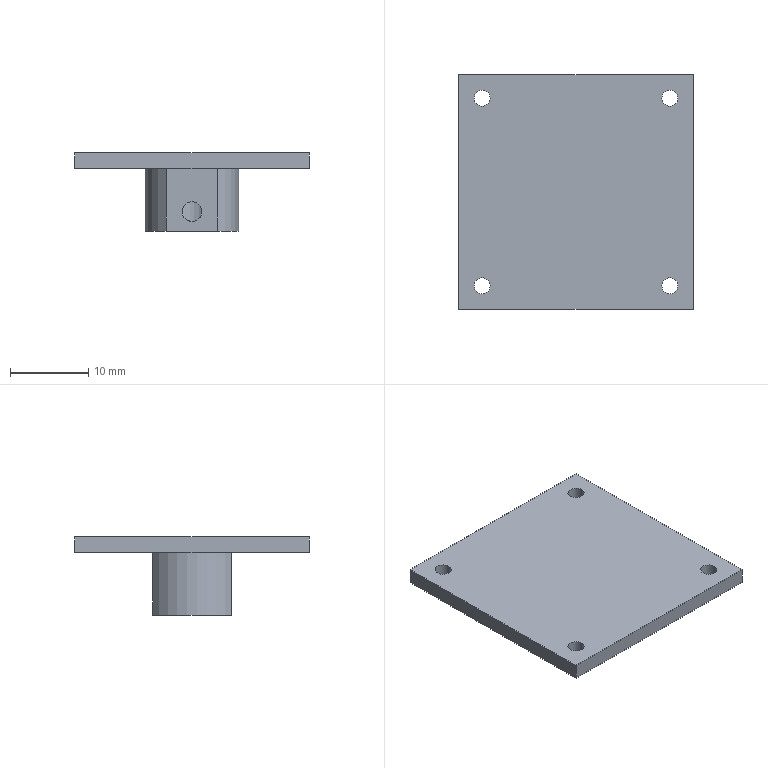Part | SolidWorks | features ICE 5, HoleWzd 2, Extrusion 1 | 1 solid | 25 faces | box 30 x 30 x 10 mm | volume 2417 mm3 | cylinder 15 | plane 10 | commonest cylinder face diameters 2.05 x8 12 x3 2.5 x2 5 x2
STEP:
#1=CARTESIAN_POINT('',(10.975,12.,0.));
#2=VERTEX_POINT('',#1);
#3=CARTESIAN_POINT('',(13.025,12.,0.));
#4=VERTEX_POINT('',#3);
#5=CARTESIAN_POINT('',(12.,12.,0.));
#6=DIRECTION('',(0.,0.,1.));
#7=DIRECTION('',(1.,0.,0.));
#8=AXIS2_PLACEMENT_3D('',#5,#6,#7);
#9=CIRCLE('',#8,1.025);
#10=EDGE_CURVE('',#2,#4,#9,.T.);
#11=ORIENTED_EDGE('',*,*,#10,.F.);
#12=CARTESIAN_POINT('',(10.975,12.,2.));
#13=VERTEX_POINT('',#12);
#14=CARTESIAN_POINT('',(10.975,12.,2.));
#15=DIRECTION('',(0.,0.,1.));
#16=VECTOR('',#15,1000.);
#17=LINE('',#14,#16);
#18=EDGE_CURVE('',#2,#13,#17,.T.);
#19=ORIENTED_EDGE('',*,*,#18,.T.);
#20=CARTESIAN_POINT('',(13.025,12.,2.));
#21=VERTEX_POINT('',#20);
#22=CARTESIAN_POINT('',(12.,12.,2.));
#23=DIRECTION('',(0.,0.,1.));
#24=DIRECTION('',(1.,0.,0.));
#25=AXIS2_PLACEMENT_3D('',#22,#23,#24);
#26=CIRCLE('',#25,1.025);
#27=EDGE_CURVE('',#13,#21,#26,.T.);
#28=ORIENTED_EDGE('',*,*,#27,.T.);
#29=CARTESIAN_POINT('',(13.025,12.,2.));
#30=DIRECTION('',(0.,0.,1.));
#31=VECTOR('',#30,1000.);
#32=LINE('',#29,#31);
#33=EDGE_CURVE('',#4,#21,#32,.T.);
#34=ORIENTED_EDGE('',*,*,#33,.F.);
#35=EDGE_LOOP('',(#11,#19,#28,#34));
#36=FACE_OUTER_BOUND('',#35,.T.);
#37=CARTESIAN_POINT('',(12.,12.,2.));
#38=DIRECTION('',(0.,0.,1.));
#39=DIRECTION('',(1.,0.,0.));
#40=AXIS2_PLACEMENT_3D('',#37,#38,#39);
#41=CYLINDRICAL_SURFACE('',#40,1.025);
#42=ADVANCED_FACE('',(#36),#41,.F.);
#43=CARTESIAN_POINT('',(10.975,-12.,0.));
#44=VERTEX_POINT('',#43);
#45=CARTESIAN_POINT('',(13.025,-12.,0.));
#46=VERTEX_POINT('',#45);
#47=CARTESIAN_POINT('',(12.,-12.,0.));
#48=DIRECTION('',(0.,0.,1.));
#49=DIRECTION('',(1.,0.,0.));
#50=AXIS2_PLACEMENT_3D('',#47,#48,#49);
#51=CIRCLE('',#50,1.025);
#52=EDGE_CURVE('',#44,#46,#51,.T.);
#53=ORIENTED_EDGE('',*,*,#52,.F.);
#54=CARTESIAN_POINT('',(10.975,-12.,2.));
#55=VERTEX_POINT('',#54);
#56=CARTESIAN_POINT('',(10.975,-12.,2.));
#57=DIRECTION('',(0.,0.,1.));
#58=VECTOR('',#57,1000.);
#59=LINE('',#56,#58);
#60=EDGE_CURVE('',#44,#55,#59,.T.);
#61=ORIENTED_EDGE('',*,*,#60,.T.);
#62=CARTESIAN_POINT('',(13.025,-12.,2.));
#63=VERTEX_POINT('',#62);
#64=CARTESIAN_POINT('',(12.,-12.,2.));
#65=DIRECTION('',(0.,0.,1.));
#66=DIRECTION('',(1.,0.,0.));
#67=AXIS2_PLACEMENT_3D('',#64,#65,#66);
#68=CIRCLE('',#67,1.025);
#69=EDGE_CURVE('',#55,#63,#68,.T.);
#70=ORIENTED_EDGE('',*,*,#69,.T.);
#71=CARTESIAN_POINT('',(13.025,-12.,2.));
#72=DIRECTION('',(0.,0.,1.));
#73=VECTOR('',#72,1000.);
#74=LINE('',#71,#73);
#75=EDGE_CURVE('',#46,#63,#74,.T.);
#76=ORIENTED_EDGE('',*,*,#75,.F.);
#77=EDGE_LOOP('',(#53,#61,#70,#76));
#78=FACE_OUTER_BOUND('',#77,.T.);
#79=CARTESIAN_POINT('',(12.,-12.,2.));
#80=DIRECTION('',(0.,0.,1.));
#81=DIRECTION('',(1.,0.,0.));
#82=AXIS2_PLACEMENT_3D('',#79,#80,#81);
#83=CYLINDRICAL_SURFACE('',#82,1.025);
#84=ADVANCED_FACE('',(#78),#83,.F.);
#85=CARTESIAN_POINT('',(-13.025,-12.,0.));
#86=VERTEX_POINT('',#85);
#87=CARTESIAN_POINT('',(-10.975,-12.,0.));
#88=VERTEX_POINT('',#87);
#89=CARTESIAN_POINT('',(-12.,-12.,0.));
#90=DIRECTION('',(0.,0.,1.));
#91=DIRECTION('',(1.,0.,0.));
#92=AXIS2_PLACEMENT_3D('',#89,#90,#91);
#93=CIRCLE('',#92,1.025);
#94=EDGE_CURVE('',#86,#88,#93,.T.);
#95=ORIENTED_EDGE('',*,*,#94,.F.);
#96=CARTESIAN_POINT('',(-13.025,-12.,2.));
#97=VERTEX_POINT('',#96);
#98=CARTESIAN_POINT('',(-13.025,-12.,2.));
#99=DIRECTION('',(0.,0.,1.));
#100=VECTOR('',#99,1000.);
#101=LINE('',#98,#100);
#102=EDGE_CURVE('',#86,#97,#101,.T.);
#103=ORIENTED_EDGE('',*,*,#102,.T.);
#104=CARTESIAN_POINT('',(-10.975,-12.,2.));
#105=VERTEX_POINT('',#104);
#106=CARTESIAN_POINT('',(-12.,-12.,2.));
#107=DIRECTION('',(0.,0.,1.));
#108=DIRECTION('',(1.,0.,0.));
#109=AXIS2_PLACEMENT_3D('',#106,#107,#108);
#110=CIRCLE('',#109,1.025);
#111=EDGE_CURVE('',#97,#105,#110,.T.);
#112=ORIENTED_EDGE('',*,*,#111,.T.);
#113=CARTESIAN_POINT('',(-10.975,-12.,2.));
#114=DIRECTION('',(0.,0.,1.));
#115=VECTOR('',#114,1000.);
#116=LINE('',#113,#115);
#117=EDGE_CURVE('',#88,#105,#116,.T.);
#118=ORIENTED_EDGE('',*,*,#117,.F.);
#119=EDGE_LOOP('',(#95,#103,#112,#118));
#120=FACE_OUTER_BOUND('',#119,.T.);
#121=CARTESIAN_POINT('',(-12.,-12.,2.));
#122=DIRECTION('',(0.,0.,1.));
#123=DIRECTION('',(1.,0.,0.));
#124=AXIS2_PLACEMENT_3D('',#121,#122,#123);
#125=CYLINDRICAL_SURFACE('',#124,1.025);
#126=ADVANCED_FACE('',(#120),#125,.F.);
#127=CARTESIAN_POINT('',(-13.025,12.,0.));
#128=VERTEX_POINT('',#127);
#129=CARTESIAN_POINT('',(-10.975,12.,0.));
#130=VERTEX_POINT('',#129);
#131=CARTESIAN_POINT('',(-12.,12.,0.));
#132=DIRECTION('',(0.,0.,1.));
#133=DIRECTION('',(1.,0.,0.));
#134=AXIS2_PLACEMENT_3D('',#131,#132,#133);
#135=CIRCLE('',#134,1.025);
#136=EDGE_CURVE('',#128,#130,#135,.T.);
#137=ORIENTED_EDGE('',*,*,#136,.F.);
#138=CARTESIAN_POINT('',(-13.025,12.,2.));
#139=VERTEX_POINT('',#138);
#140=CARTESIAN_POINT('',(-13.025,12.,2.));
#141=DIRECTION('',(0.,0.,1.));
#142=VECTOR('',#141,1000.);
#143=LINE('',#140,#142);
#144=EDGE_CURVE('',#128,#139,#143,.T.);
#145=ORIENTED_EDGE('',*,*,#144,.T.);
#146=CARTESIAN_POINT('',(-10.975,12.,2.));
#147=VERTEX_POINT('',#146);
#148=CARTESIAN_POINT('',(-12.,12.,2.));
#149=DIRECTION('',(0.,0.,1.));
#150=DIRECTION('',(1.,0.,0.));
#151=AXIS2_PLACEMENT_3D('',#148,#149,#150);
#152=CIRCLE('',#151,1.025);
#153=EDGE_CURVE('',#139,#147,#152,.T.);
#154=ORIENTED_EDGE('',*,*,#153,.T.);
#155=CARTESIAN_POINT('',(-10.975,12.,2.));
#156=DIRECTION('',(0.,0.,1.));
#157=VECTOR('',#156,1000.);
#158=LINE('',#155,#157);
#159=EDGE_CURVE('',#130,#147,#158,.T.);
#160=ORIENTED_EDGE('',*,*,#159,.F.);
#161=EDGE_LOOP('',(#137,#145,#154,#160));
#162=FACE_OUTER_BOUND('',#161,.T.);
#163=CARTESIAN_POINT('',(-12.,12.,2.));
#164=DIRECTION('',(0.,0.,1.));
#165=DIRECTION('',(1.,0.,0.));
#166=AXIS2_PLACEMENT_3D('',#163,#164,#165);
#167=CYLINDRICAL_SURFACE('',#166,1.025);
#168=ADVANCED_FACE('',(#162),#167,.F.);
#169=CARTESIAN_POINT('',(0.,-2.5,-4.25));
#170=VERTEX_POINT('',#169);
#171=CARTESIAN_POINT('',(0.,-2.5,-6.75));
#172=VERTEX_POINT('',#171);
#173=CARTESIAN_POINT('',(0.,-2.5,-4.25));
#174=CARTESIAN_POINT('',(-0.08285,-2.5,-4.25));
#175=CARTESIAN_POINT('',(-0.1672,-2.496,-4.258));
#176=CARTESIAN_POINT('',(-0.3292,-2.48,-4.291));
#177=CARTESIAN_POINT('',(-0.4077,-2.468,-4.315));
#178=CARTESIAN_POINT('',(-0.6361,-2.423,-4.411));
#179=CARTESIAN_POINT('',(-0.7717,-2.381,-4.504));
#180=CARTESIAN_POINT('',(-0.9986,-2.295,-4.731));
#181=CARTESIAN_POINT('',(-1.09,-2.251,-4.868));
#182=CARTESIAN_POINT('',(-1.216,-2.186,-5.167));
#183=CARTESIAN_POINT('',(-1.25,-2.165,-5.333));
#184=CARTESIAN_POINT('',(-1.25,-2.165,-5.664));
#185=CARTESIAN_POINT('',(-1.217,-2.185,-5.831));
#186=CARTESIAN_POINT('',(-1.09,-2.251,-6.133));
#187=CARTESIAN_POINT('',(-0.9987,-2.295,-6.269));
#188=CARTESIAN_POINT('',(-0.8277,-2.36,-6.44));
#189=CARTESIAN_POINT('',(-0.7659,-2.381,-6.491));
#190=CARTESIAN_POINT('',(-0.6321,-2.42,-6.581));
#191=CARTESIAN_POINT('',(-0.5593,-2.438,-6.621));
#192=CARTESIAN_POINT('',(-0.3335,-2.482,-6.716));
#193=CARTESIAN_POINT('',(-0.168,-2.5,-6.75));
#194=CARTESIAN_POINT('',(0.,-2.5,-6.75));
#195=B_SPLINE_CURVE_WITH_KNOTS('',3,(#173,#174,#175,#176,#177,#178,#179,#180,#181,#182,#183,#184,#185,#186,#187,#188,#189,#190,#191,#192,#193,#194),.UNSPECIFIED.,.F.,.F.,(4,2,2,2,2,2,2,2,2,2,4),(0.003976,0.004224,0.004472,0.004969,0.005465,0.005961,0.006457,0.006953,0.007201,0.007449,0.007946),.UNSPECIFIED.);
#196=EDGE_CURVE('',#170,#172,#195,.T.);
#197=ORIENTED_EDGE('',*,*,#196,.F.);
#198=CARTESIAN_POINT('',(0.,-5.,-4.25));
#199=VERTEX_POINT('',#198);
#200=CARTESIAN_POINT('',(0.,-5.,-4.25));
#201=DIRECTION('',(0.,-1.,0.));
#202=VECTOR('',#201,1000.);
#203=LINE('',#200,#202);
#204=EDGE_CURVE('',#170,#199,#203,.T.);
#205=ORIENTED_EDGE('',*,*,#204,.T.);
#206=CARTESIAN_POINT('',(0.,-5.,-6.75));
#207=VERTEX_POINT('',#206);
#208=CARTESIAN_POINT('',(0.,-5.,-5.5));
#209=DIRECTION('',(0.,-1.,0.));
#210=DIRECTION('',(0.,0.,-1.));
#211=AXIS2_PLACEMENT_3D('',#208,#209,#210);
#212=CIRCLE('',#211,1.25);
#213=EDGE_CURVE('',#199,#207,#212,.T.);
#214=ORIENTED_EDGE('',*,*,#213,.T.);
#215=CARTESIAN_POINT('',(0.,-5.,-6.75));
#216=DIRECTION('',(0.,-1.,0.));
#217=VECTOR('',#216,1000.);
#218=LINE('',#215,#217);
#219=EDGE_CURVE('',#172,#207,#218,.T.);
#220=ORIENTED_EDGE('',*,*,#219,.F.);
#221=EDGE_LOOP('',(#197,#205,#214,#220));
#222=FACE_OUTER_BOUND('',#221,.T.);
#223=CARTESIAN_POINT('',(0.,-5.,-5.5));
#224=DIRECTION('',(0.,-1.,0.));
#225=DIRECTION('',(0.,0.,-1.));
#226=AXIS2_PLACEMENT_3D('',#223,#224,#225);
#227=CYLINDRICAL_SURFACE('',#226,1.25);
#228=ADVANCED_FACE('',(#222),#227,.F.);
#229=CARTESIAN_POINT('',(0.,-2.5,-6.75));
#230=CARTESIAN_POINT('',(0.08412,-2.5,-6.75));
#231=CARTESIAN_POINT('',(0.1666,-2.496,-6.742));
#232=CARTESIAN_POINT('',(0.3284,-2.48,-6.709));
#233=CARTESIAN_POINT('',(0.4085,-2.468,-6.684));
#234=CARTESIAN_POINT('',(0.635,-2.423,-6.589));
#235=CARTESIAN_POINT('',(0.7717,-2.381,-6.496));
#236=CARTESIAN_POINT('',(0.9981,-2.295,-6.269));
#237=CARTESIAN_POINT('',(1.09,-2.251,-6.133));
#238=CARTESIAN_POINT('',(1.184,-2.202,-5.908));
#239=CARTESIAN_POINT('',(1.209,-2.188,-5.828));
#240=CARTESIAN_POINT('',(1.242,-2.17,-5.666));
#241=CARTESIAN_POINT('',(1.25,-2.165,-5.584));
#242=CARTESIAN_POINT('',(1.25,-2.165,-5.335));
#243=CARTESIAN_POINT('',(1.216,-2.185,-5.168));
#244=CARTESIAN_POINT('',(1.089,-2.251,-4.866));
#245=CARTESIAN_POINT('',(0.9974,-2.296,-4.73));
#246=CARTESIAN_POINT('',(0.7706,-2.381,-4.503));
#247=CARTESIAN_POINT('',(0.6332,-2.423,-4.41));
#248=CARTESIAN_POINT('',(0.3331,-2.482,-4.284));
#249=CARTESIAN_POINT('',(0.166,-2.5,-4.25));
#250=CARTESIAN_POINT('',(0.,-2.5,-4.25));
#251=B_SPLINE_CURVE_WITH_KNOTS('',3,(#229,#230,#231,#232,#233,#234,#235,#236,#237,#238,#239,#240,#241,#242,#243,#244,#245,#246,#247,#248,#249,#250),.UNSPECIFIED.,.F.,.F.,(4,2,2,2,2,2,2,2,2,2,4),(0.,0.0002485,0.000497,0.0009941,0.001491,0.00174,0.001988,0.002485,0.002982,0.003479,0.003976),.UNSPECIFIED.);
#252=EDGE_CURVE('',#172,#170,#251,.T.);
#253=ORIENTED_EDGE('',*,*,#252,.T.);
#254=ORIENTED_EDGE('',*,*,#196,.T.);
#255=EDGE_LOOP('',(#253,#254));
#256=FACE_BOUND('',#255,.T.);
#257=CARTESIAN_POINT('',(2.5,0.,1.));
#258=VERTEX_POINT('',#257);
#259=CARTESIAN_POINT('',(-2.5,0.,1.));
#260=VERTEX_POINT('',#259);
#261=CARTESIAN_POINT('',(0.,0.,1.));
#262=DIRECTION('',(0.,0.,-1.));
#263=DIRECTION('',(-1.,0.,0.));
#264=AXIS2_PLACEMENT_3D('',#261,#262,#263);
#265=CIRCLE('',#264,2.5);
#266=EDGE_CURVE('',#258,#260,#265,.T.);
#267=ORIENTED_EDGE('',*,*,#266,.F.);
#268=CARTESIAN_POINT('',(2.5,0.,-8.));
#269=VERTEX_POINT('',#268);
#270=CARTESIAN_POINT('',(2.5,0.,1.));
#271=DIRECTION('',(0.,0.,-1.));
#272=VECTOR('',#271,1000.);
#273=LINE('',#270,#272);
#274=EDGE_CURVE('',#258,#269,#273,.T.);
#275=ORIENTED_EDGE('',*,*,#274,.T.);
#276=CARTESIAN_POINT('',(-2.5,0.,-8.));
#277=VERTEX_POINT('',#276);
#278=CARTESIAN_POINT('',(0.,0.,-8.));
#279=DIRECTION('',(0.,0.,-1.));
#280=DIRECTION('',(-1.,0.,0.));
#281=AXIS2_PLACEMENT_3D('',#278,#279,#280);
#282=CIRCLE('',#281,2.5);
#283=EDGE_CURVE('',#269,#277,#282,.T.);
#284=ORIENTED_EDGE('',*,*,#283,.T.);
#285=CARTESIAN_POINT('',(-2.5,0.,1.));
#286=DIRECTION('',(0.,0.,-1.));
#287=VECTOR('',#286,1000.);
#288=LINE('',#285,#287);
#289=EDGE_CURVE('',#260,#277,#288,.T.);
#290=ORIENTED_EDGE('',*,*,#289,.F.);
#291=EDGE_LOOP('',(#267,#275,#284,#290));
#292=FACE_OUTER_BOUND('',#291,.T.);
#293=CARTESIAN_POINT('',(0.,0.,1.));
#294=DIRECTION('',(0.,0.,-1.));
#295=DIRECTION('',(-1.,0.,0.));
#296=AXIS2_PLACEMENT_3D('',#293,#294,#295);
#297=CYLINDRICAL_SURFACE('',#296,2.5);
#298=ADVANCED_FACE('',(#256,#292),#297,.F.);
#299=CARTESIAN_POINT('',(6.,0.,-8.));
#300=VERTEX_POINT('',#299);
#301=CARTESIAN_POINT('',(3.317,-5.,-8.));
#302=VERTEX_POINT('',#301);
#303=CARTESIAN_POINT('',(0.,0.,-8.));
#304=DIRECTION('',(0.,0.,-1.));
#305=DIRECTION('',(-1.,0.,0.));
#306=AXIS2_PLACEMENT_3D('',#303,#304,#305);
#307=CIRCLE('',#306,6.);
#308=EDGE_CURVE('',#300,#302,#307,.T.);
#309=ORIENTED_EDGE('',*,*,#308,.F.);
#310=CARTESIAN_POINT('',(6.,0.,0.));
#311=VERTEX_POINT('',#310);
#312=CARTESIAN_POINT('',(6.,0.,-8.));
#313=DIRECTION('',(0.,0.,1.));
#314=VECTOR('',#313,1000.);
#315=LINE('',#312,#314);
#316=EDGE_CURVE('',#300,#311,#315,.T.);
#317=ORIENTED_EDGE('',*,*,#316,.T.);
#318=CARTESIAN_POINT('',(3.317,-5.,0.));
#319=VERTEX_POINT('',#318);
#320=CARTESIAN_POINT('',(0.,0.,0.));
#321=DIRECTION('',(0.,0.,-1.));
#322=DIRECTION('',(-1.,0.,0.));
#323=AXIS2_PLACEMENT_3D('',#320,#321,#322);
#324=CIRCLE('',#323,6.);
#325=EDGE_CURVE('',#311,#319,#324,.T.);
#326=ORIENTED_EDGE('',*,*,#325,.T.);
#327=CARTESIAN_POINT('',(3.317,-5.,-8.));
#328=DIRECTION('',(0.,0.,1.));
#329=VECTOR('',#328,1000.);
#330=LINE('',#327,#329);
#331=EDGE_CURVE('',#302,#319,#330,.T.);
#332=ORIENTED_EDGE('',*,*,#331,.F.);
#333=EDGE_LOOP('',(#309,#317,#326,#332));
#334=FACE_OUTER_BOUND('',#333,.T.);
#335=CARTESIAN_POINT('',(0.,0.,-8.));
#336=DIRECTION('',(0.,0.,1.));
#337=DIRECTION('',(1.,0.,0.));
#338=AXIS2_PLACEMENT_3D('',#335,#336,#337);
#339=CYLINDRICAL_SURFACE('',#338,6.);
#340=ADVANCED_FACE('',(#334),#339,.T.);
#341=ORIENTED_EDGE('',*,*,#316,.F.);
#342=CARTESIAN_POINT('',(3.317,5.,-8.));
#343=VERTEX_POINT('',#342);
#344=CARTESIAN_POINT('',(0.,0.,-8.));
#345=DIRECTION('',(0.,0.,-1.));
#346=DIRECTION('',(-1.,0.,0.));
#347=AXIS2_PLACEMENT_3D('',#344,#345,#346);
#348=CIRCLE('',#347,6.);
#349=EDGE_CURVE('',#343,#300,#348,.T.);
#350=ORIENTED_EDGE('',*,*,#349,.F.);
#351=CARTESIAN_POINT('',(3.317,5.,0.));
#352=VERTEX_POINT('',#351);
#353=CARTESIAN_POINT('',(3.317,5.,-8.));
#354=DIRECTION('',(0.,0.,-1.));
#355=VECTOR('',#354,1000.);
#356=LINE('',#353,#355);
#357=EDGE_CURVE('',#352,#343,#356,.T.);
#358=ORIENTED_EDGE('',*,*,#357,.F.);
#359=CARTESIAN_POINT('',(0.,0.,0.));
#360=DIRECTION('',(0.,0.,-1.));
#361=DIRECTION('',(-1.,0.,0.));
#362=AXIS2_PLACEMENT_3D('',#359,#360,#361);
#363=CIRCLE('',#362,6.);
#364=EDGE_CURVE('',#352,#311,#363,.T.);
#365=ORIENTED_EDGE('',*,*,#364,.T.);
#366=EDGE_LOOP('',(#341,#350,#358,#365));
#367=FACE_OUTER_BOUND('',#366,.T.);
#368=CARTESIAN_POINT('',(0.,0.,-8.));
#369=DIRECTION('',(0.,0.,1.));
#370=DIRECTION('',(1.,0.,0.));
#371=AXIS2_PLACEMENT_3D('',#368,#369,#370);
#372=CYLINDRICAL_SURFACE('',#371,6.);
#373=ADVANCED_FACE('',(#367),#372,.T.);
#374=CARTESIAN_POINT('',(-3.317,-5.,0.));
#375=VERTEX_POINT('',#374);
#376=CARTESIAN_POINT('',(-3.317,-5.,-8.));
#377=VERTEX_POINT('',#376);
#378=CARTESIAN_POINT('',(-3.317,-5.,-8.));
#379=DIRECTION('',(0.,0.,-1.));
#380=VECTOR('',#379,1000.);
#381=LINE('',#378,#380);
#382=EDGE_CURVE('',#375,#377,#381,.T.);
#383=ORIENTED_EDGE('',*,*,#382,.F.);
#384=CARTESIAN_POINT('',(-3.317,5.,0.));
#385=VERTEX_POINT('',#384);
#386=CARTESIAN_POINT('',(0.,0.,0.));
#387=DIRECTION('',(0.,0.,-1.));
#388=DIRECTION('',(-1.,0.,0.));
#389=AXIS2_PLACEMENT_3D('',#386,#387,#388);
#390=CIRCLE('',#389,6.);
#391=EDGE_CURVE('',#375,#385,#390,.T.);
#392=ORIENTED_EDGE('',*,*,#391,.T.);
#393=CARTESIAN_POINT('',(-3.317,5.,-8.));
#394=VERTEX_POINT('',#393);
#395=CARTESIAN_POINT('',(-3.317,5.,-8.));
#396=DIRECTION('',(0.,0.,1.));
#397=VECTOR('',#396,1000.);
#398=LINE('',#395,#397);
#399=EDGE_CURVE('',#394,#385,#398,.T.);
#400=ORIENTED_EDGE('',*,*,#399,.F.);
#401=CARTESIAN_POINT('',(0.,0.,-8.));
#402=DIRECTION('',(0.,0.,-1.));
#403=DIRECTION('',(-1.,0.,0.));
#404=AXIS2_PLACEMENT_3D('',#401,#402,#403);
#405=CIRCLE('',#404,6.);
#406=EDGE_CURVE('',#377,#394,#405,.T.);
#407=ORIENTED_EDGE('',*,*,#406,.F.);
#408=EDGE_LOOP('',(#383,#392,#400,#407));
#409=FACE_OUTER_BOUND('',#408,.T.);
#410=CARTESIAN_POINT('',(0.,0.,-8.));
#411=DIRECTION('',(0.,0.,1.));
#412=DIRECTION('',(1.,0.,0.));
#413=AXIS2_PLACEMENT_3D('',#410,#411,#412);
#414=CYLINDRICAL_SURFACE('',#413,6.);
#415=ADVANCED_FACE('',(#409),#414,.T.);
#416=CARTESIAN_POINT('',(0.,0.,-8.));
#417=DIRECTION('',(0.,0.,-1.));
#418=DIRECTION('',(-1.,0.,0.));
#419=AXIS2_PLACEMENT_3D('',#416,#417,#418);
#420=CIRCLE('',#419,2.5);
#421=EDGE_CURVE('',#277,#269,#420,.T.);
#422=ORIENTED_EDGE('',*,*,#421,.F.);
#423=ORIENTED_EDGE('',*,*,#283,.F.);
#424=EDGE_LOOP('',(#422,#423));
#425=FACE_BOUND('',#424,.T.);
#426=ORIENTED_EDGE('',*,*,#349,.T.);
#427=ORIENTED_EDGE('',*,*,#308,.T.);
#428=CARTESIAN_POINT('',(0.,-5.,-8.));
#429=DIRECTION('',(-1.,0.,0.));
#430=VECTOR('',#429,1000.);
#431=LINE('',#428,#430);
#432=EDGE_CURVE('',#302,#377,#431,.T.);
#433=ORIENTED_EDGE('',*,*,#432,.T.);
#434=ORIENTED_EDGE('',*,*,#406,.T.);
#435=CARTESIAN_POINT('',(0.,5.,-8.));
#436=DIRECTION('',(1.,0.,0.));
#437=VECTOR('',#436,1000.);
#438=LINE('',#435,#437);
#439=EDGE_CURVE('',#394,#343,#438,.T.);
#440=ORIENTED_EDGE('',*,*,#439,.T.);
#441=EDGE_LOOP('',(#426,#427,#433,#434,#440));
#442=FACE_OUTER_BOUND('',#441,.T.);
#443=CARTESIAN_POINT('',(0.,0.,-8.));
#444=DIRECTION('',(0.,0.,-1.));
#445=DIRECTION('',(-1.,0.,0.));
#446=AXIS2_PLACEMENT_3D('',#443,#444,#445);
#447=PLANE('',#446);
#448=ADVANCED_FACE('',(#425,#442),#447,.T.);
#449=CARTESIAN_POINT('',(15.,-15.,0.));
#450=VERTEX_POINT('',#449);
#451=CARTESIAN_POINT('',(15.,15.,0.));
#452=VERTEX_POINT('',#451);
#453=CARTESIAN_POINT('',(15.,15.,0.));
#454=DIRECTION('',(0.,1.,0.));
#455=VECTOR('',#454,1000.);
#456=LINE('',#453,#455);
#457=EDGE_CURVE('',#450,#452,#456,.T.);
#458=ORIENTED_EDGE('',*,*,#457,.T.);
#459=CARTESIAN_POINT('',(15.,15.,2.));
#460=VERTEX_POINT('',#459);
#461=CARTESIAN_POINT('',(15.,15.,2.));
#462=DIRECTION('',(0.,0.,-1.));
#463=VECTOR('',#462,1000.);
#464=LINE('',#461,#463);
#465=EDGE_CURVE('',#460,#452,#464,.T.);
#466=ORIENTED_EDGE('',*,*,#465,.F.);
#467=CARTESIAN_POINT('',(15.,-15.,2.));
#468=VERTEX_POINT('',#467);
#469=CARTESIAN_POINT('',(15.,15.,2.));
#470=DIRECTION('',(0.,1.,0.));
#471=VECTOR('',#470,1000.);
#472=LINE('',#469,#471);
#473=EDGE_CURVE('',#468,#460,#472,.T.);
#474=ORIENTED_EDGE('',*,*,#473,.F.);
#475=CARTESIAN_POINT('',(15.,-15.,2.));
#476=DIRECTION('',(0.,0.,-1.));
#477=VECTOR('',#476,1000.);
#478=LINE('',#475,#477);
#479=EDGE_CURVE('',#468,#450,#478,.T.);
#480=ORIENTED_EDGE('',*,*,#479,.T.);
#481=EDGE_LOOP('',(#458,#466,#474,#480));
#482=FACE_OUTER_BOUND('',#481,.T.);
#483=CARTESIAN_POINT('',(15.,15.,2.));
#484=DIRECTION('',(-1.,0.,0.));
#485=DIRECTION('',(0.,0.,1.));
#486=AXIS2_PLACEMENT_3D('',#483,#484,#485);
#487=PLANE('',#486);
#488=ADVANCED_FACE('',(#482),#487,.F.);
#489=CARTESIAN_POINT('',(-15.,15.,0.));
#490=VERTEX_POINT('',#489);
#491=CARTESIAN_POINT('',(-15.,15.,0.));
#492=DIRECTION('',(-1.,0.,0.));
#493=VECTOR('',#492,1000.);
#494=LINE('',#491,#493);
#495=EDGE_CURVE('',#452,#490,#494,.T.);
#496=ORIENTED_EDGE('',*,*,#495,.T.);
#497=CARTESIAN_POINT('',(-15.,15.,2.));
#498=VERTEX_POINT('',#497);
#499=CARTESIAN_POINT('',(-15.,15.,2.));
#500=DIRECTION('',(0.,0.,-1.));
#501=VECTOR('',#500,1000.);
#502=LINE('',#499,#501);
#503=EDGE_CURVE('',#498,#490,#502,.T.);
#504=ORIENTED_EDGE('',*,*,#503,.F.);
#505=CARTESIAN_POINT('',(-15.,15.,2.));
#506=DIRECTION('',(-1.,0.,0.));
#507=VECTOR('',#506,1000.);
#508=LINE('',#505,#507);
#509=EDGE_CURVE('',#460,#498,#508,.T.);
#510=ORIENTED_EDGE('',*,*,#509,.F.);
#511=ORIENTED_EDGE('',*,*,#465,.T.);
#512=EDGE_LOOP('',(#496,#504,#510,#511));
#513=FACE_OUTER_BOUND('',#512,.T.);
#514=CARTESIAN_POINT('',(-15.,15.,2.));
#515=DIRECTION('',(0.,-1.,0.));
#516=DIRECTION('',(0.,0.,-1.));
#517=AXIS2_PLACEMENT_3D('',#514,#515,#516);
#518=PLANE('',#517);
#519=ADVANCED_FACE('',(#513),#518,.F.);
#520=CARTESIAN_POINT('',(-15.,-15.,0.));
#521=VERTEX_POINT('',#520);
#522=CARTESIAN_POINT('',(-15.,15.,0.));
#523=DIRECTION('',(0.,-1.,0.));
#524=VECTOR('',#523,1000.);
#525=LINE('',#522,#524);
#526=EDGE_CURVE('',#490,#521,#525,.T.);
#527=ORIENTED_EDGE('',*,*,#526,.T.);
#528=CARTESIAN_POINT('',(-15.,-15.,2.));
#529=VERTEX_POINT('',#528);
#530=CARTESIAN_POINT('',(-15.,-15.,2.));
#531=DIRECTION('',(0.,0.,-1.));
#532=VECTOR('',#531,1000.);
#533=LINE('',#530,#532);
#534=EDGE_CURVE('',#529,#521,#533,.T.);
#535=ORIENTED_EDGE('',*,*,#534,.F.);
#536=CARTESIAN_POINT('',(-15.,15.,2.));
#537=DIRECTION('',(0.,-1.,0.));
#538=VECTOR('',#537,1000.);
#539=LINE('',#536,#538);
#540=EDGE_CURVE('',#498,#529,#539,.T.);
#541=ORIENTED_EDGE('',*,*,#540,.F.);
#542=ORIENTED_EDGE('',*,*,#503,.T.);
#543=EDGE_LOOP('',(#527,#535,#541,#542));
#544=FACE_OUTER_BOUND('',#543,.T.);
#545=CARTESIAN_POINT('',(-15.,15.,2.));
#546=DIRECTION('',(1.,0.,0.));
#547=DIRECTION('',(0.,0.,-1.));
#548=AXIS2_PLACEMENT_3D('',#545,#546,#547);
#549=PLANE('',#548);
#550=ADVANCED_FACE('',(#544),#549,.F.);
#551=CARTESIAN_POINT('',(-15.,-15.,0.));
#552=DIRECTION('',(1.,0.,0.));
#553=VECTOR('',#552,1000.);
#554=LINE('',#551,#553);
#555=EDGE_CURVE('',#521,#450,#554,.T.);
#556=ORIENTED_EDGE('',*,*,#555,.T.);
#557=ORIENTED_EDGE('',*,*,#479,.F.);
#558=CARTESIAN_POINT('',(-15.,-15.,2.));
#559=DIRECTION('',(1.,0.,0.));
#560=VECTOR('',#559,1000.);
#561=LINE('',#558,#560);
#562=EDGE_CURVE('',#529,#468,#561,.T.);
#563=ORIENTED_EDGE('',*,*,#562,.F.);
#564=ORIENTED_EDGE('',*,*,#534,.T.);
#565=EDGE_LOOP('',(#556,#557,#563,#564));
#566=FACE_OUTER_BOUND('',#565,.T.);
#567=CARTESIAN_POINT('',(-15.,-15.,2.));
#568=DIRECTION('',(0.,1.,0.));
#569=DIRECTION('',(0.,0.,1.));
#570=AXIS2_PLACEMENT_3D('',#567,#568,#569);
#571=PLANE('',#570);
#572=ADVANCED_FACE('',(#566),#571,.F.);
#573=CARTESIAN_POINT('',(12.,12.,2.));
#574=DIRECTION('',(0.,0.,1.));
#575=DIRECTION('',(1.,0.,0.));
#576=AXIS2_PLACEMENT_3D('',#573,#574,#575);
#577=CIRCLE('',#576,1.025);
#578=EDGE_CURVE('',#21,#13,#577,.T.);
#579=ORIENTED_EDGE('',*,*,#578,.F.);
#580=ORIENTED_EDGE('',*,*,#27,.F.);
#581=EDGE_LOOP('',(#579,#580));
#582=FACE_BOUND('',#581,.T.);
#583=CARTESIAN_POINT('',(12.,-12.,2.));
#584=DIRECTION('',(0.,0.,1.));
#585=DIRECTION('',(1.,0.,0.));
#586=AXIS2_PLACEMENT_3D('',#583,#584,#585);
#587=CIRCLE('',#586,1.025);
#588=EDGE_CURVE('',#63,#55,#587,.T.);
#589=ORIENTED_EDGE('',*,*,#588,.F.);
#590=ORIENTED_EDGE('',*,*,#69,.F.);
#591=EDGE_LOOP('',(#589,#590));
#592=FACE_BOUND('',#591,.T.);
#593=CARTESIAN_POINT('',(-12.,-12.,2.));
#594=DIRECTION('',(0.,0.,1.));
#595=DIRECTION('',(1.,0.,0.));
#596=AXIS2_PLACEMENT_3D('',#593,#594,#595);
#597=CIRCLE('',#596,1.025);
#598=EDGE_CURVE('',#105,#97,#597,.T.);
#599=ORIENTED_EDGE('',*,*,#598,.F.);
#600=ORIENTED_EDGE('',*,*,#111,.F.);
#601=EDGE_LOOP('',(#599,#600));
#602=FACE_BOUND('',#601,.T.);
#603=CARTESIAN_POINT('',(-12.,12.,2.));
#604=DIRECTION('',(0.,0.,1.));
#605=DIRECTION('',(1.,0.,0.));
#606=AXIS2_PLACEMENT_3D('',#603,#604,#605);
#607=CIRCLE('',#606,1.025);
#608=EDGE_CURVE('',#147,#139,#607,.T.);
#609=ORIENTED_EDGE('',*,*,#608,.F.);
#610=ORIENTED_EDGE('',*,*,#153,.F.);
#611=EDGE_LOOP('',(#609,#610));
#612=FACE_BOUND('',#611,.T.);
#613=ORIENTED_EDGE('',*,*,#473,.T.);
#614=ORIENTED_EDGE('',*,*,#509,.T.);
#615=ORIENTED_EDGE('',*,*,#540,.T.);
#616=ORIENTED_EDGE('',*,*,#562,.T.);
#617=EDGE_LOOP('',(#613,#614,#615,#616));
#618=FACE_OUTER_BOUND('',#617,.T.);
#619=CARTESIAN_POINT('',(0.,0.,2.));
#620=DIRECTION('',(0.,0.,1.));
#621=DIRECTION('',(1.,0.,0.));
#622=AXIS2_PLACEMENT_3D('',#619,#620,#621);
#623=PLANE('',#622);
#624=ADVANCED_FACE('',(#582,#592,#602,#612,#618),#623,.T.);
#625=CARTESIAN_POINT('',(12.,12.,0.));
#626=DIRECTION('',(0.,0.,1.));
#627=DIRECTION('',(1.,0.,0.));
#628=AXIS2_PLACEMENT_3D('',#625,#626,#627);
#629=CIRCLE('',#628,1.025);
#630=EDGE_CURVE('',#4,#2,#629,.T.);
#631=ORIENTED_EDGE('',*,*,#630,.T.);
#632=ORIENTED_EDGE('',*,*,#10,.T.);
#633=EDGE_LOOP('',(#631,#632));
#634=FACE_BOUND('',#633,.T.);
#635=CARTESIAN_POINT('',(12.,-12.,0.));
#636=DIRECTION('',(0.,0.,1.));
#637=DIRECTION('',(1.,0.,0.));
#638=AXIS2_PLACEMENT_3D('',#635,#636,#637);
#639=CIRCLE('',#638,1.025);
#640=EDGE_CURVE('',#46,#44,#639,.T.);
#641=ORIENTED_EDGE('',*,*,#640,.T.);
#642=ORIENTED_EDGE('',*,*,#52,.T.);
#643=EDGE_LOOP('',(#641,#642));
#644=FACE_BOUND('',#643,.T.);
#645=CARTESIAN_POINT('',(-12.,-12.,0.));
#646=DIRECTION('',(0.,0.,1.));
#647=DIRECTION('',(1.,0.,0.));
#648=AXIS2_PLACEMENT_3D('',#645,#646,#647);
#649=CIRCLE('',#648,1.025);
#650=EDGE_CURVE('',#88,#86,#649,.T.);
#651=ORIENTED_EDGE('',*,*,#650,.T.);
#652=ORIENTED_EDGE('',*,*,#94,.T.);
#653=EDGE_LOOP('',(#651,#652));
#654=FACE_BOUND('',#653,.T.);
#655=CARTESIAN_POINT('',(-12.,12.,0.));
#656=DIRECTION('',(0.,0.,1.));
#657=DIRECTION('',(1.,0.,0.));
#658=AXIS2_PLACEMENT_3D('',#655,#656,#657);
#659=CIRCLE('',#658,1.025);
#660=EDGE_CURVE('',#130,#128,#659,.T.);
#661=ORIENTED_EDGE('',*,*,#660,.T.);
#662=ORIENTED_EDGE('',*,*,#136,.T.);
#663=EDGE_LOOP('',(#661,#662));
#664=FACE_BOUND('',#663,.T.);
#665=ORIENTED_EDGE('',*,*,#391,.F.);
#666=CARTESIAN_POINT('',(7.772,-5.,0.));
#667=DIRECTION('',(-1.,0.,0.));
#668=VECTOR('',#667,1000.);
#669=LINE('',#666,#668);
#670=EDGE_CURVE('',#319,#375,#669,.T.);
#671=ORIENTED_EDGE('',*,*,#670,.F.);
#672=ORIENTED_EDGE('',*,*,#325,.F.);
#673=ORIENTED_EDGE('',*,*,#364,.F.);
#674=CARTESIAN_POINT('',(7.772,5.,0.));
#675=DIRECTION('',(1.,0.,0.));
#676=VECTOR('',#675,1000.);
#677=LINE('',#674,#676);
#678=EDGE_CURVE('',#385,#352,#677,.T.);
#679=ORIENTED_EDGE('',*,*,#678,.F.);
#680=EDGE_LOOP('',(#665,#671,#672,#673,#679));
#681=FACE_BOUND('',#680,.T.);
#682=ORIENTED_EDGE('',*,*,#457,.F.);
#683=ORIENTED_EDGE('',*,*,#555,.F.);
#684=ORIENTED_EDGE('',*,*,#526,.F.);
#685=ORIENTED_EDGE('',*,*,#495,.F.);
#686=EDGE_LOOP('',(#682,#683,#684,#685));
#687=FACE_OUTER_BOUND('',#686,.T.);
#688=CARTESIAN_POINT('',(0.,0.,0.));
#689=DIRECTION('',(0.,0.,1.));
#690=DIRECTION('',(1.,0.,0.));
#691=AXIS2_PLACEMENT_3D('',#688,#689,#690);
#692=PLANE('',#691);
#693=ADVANCED_FACE('',(#634,#644,#654,#664,#681,#687),#692,.F.);
#694=ORIENTED_EDGE('',*,*,#274,.F.);
#695=CARTESIAN_POINT('',(0.,0.,1.));
#696=DIRECTION('',(0.,0.,-1.));
#697=DIRECTION('',(-1.,0.,0.));
#698=AXIS2_PLACEMENT_3D('',#695,#696,#697);
#699=CIRCLE('',#698,2.5);
#700=EDGE_CURVE('',#260,#258,#699,.T.);
#701=ORIENTED_EDGE('',*,*,#700,.F.);
#702=ORIENTED_EDGE('',*,*,#289,.T.);
#703=ORIENTED_EDGE('',*,*,#421,.T.);
#704=EDGE_LOOP('',(#694,#701,#702,#703));
#705=FACE_OUTER_BOUND('',#704,.T.);
#706=CARTESIAN_POINT('',(0.,0.,1.));
#707=DIRECTION('',(0.,0.,-1.));
#708=DIRECTION('',(-1.,0.,0.));
#709=AXIS2_PLACEMENT_3D('',#706,#707,#708);
#710=CYLINDRICAL_SURFACE('',#709,2.5);
#711=ADVANCED_FACE('',(#705),#710,.F.);
#712=ORIENTED_EDGE('',*,*,#700,.T.);
#713=ORIENTED_EDGE('',*,*,#266,.T.);
#714=EDGE_LOOP('',(#712,#713));
#715=FACE_OUTER_BOUND('',#714,.T.);
#716=CARTESIAN_POINT('',(0.,0.,1.));
#717=DIRECTION('',(0.,0.,-1.));
#718=DIRECTION('',(-1.,0.,0.));
#719=AXIS2_PLACEMENT_3D('',#716,#717,#718);
#720=PLANE('',#719);
#721=ADVANCED_FACE('',(#715),#720,.T.);
#722=ORIENTED_EDGE('',*,*,#399,.T.);
#723=ORIENTED_EDGE('',*,*,#678,.T.);
#724=ORIENTED_EDGE('',*,*,#357,.T.);
#725=ORIENTED_EDGE('',*,*,#439,.F.);
#726=EDGE_LOOP('',(#722,#723,#724,#725));
#727=FACE_OUTER_BOUND('',#726,.T.);
#728=CARTESIAN_POINT('',(7.772,5.,0.));
#729=DIRECTION('',(0.,1.,0.));
#730=DIRECTION('',(0.,0.,1.));
#731=AXIS2_PLACEMENT_3D('',#728,#729,#730);
#732=PLANE('',#731);
#733=ADVANCED_FACE('',(#727),#732,.T.);
#734=CARTESIAN_POINT('',(0.,-5.,-5.5));
#735=DIRECTION('',(0.,-1.,0.));
#736=DIRECTION('',(0.,0.,-1.));
#737=AXIS2_PLACEMENT_3D('',#734,#735,#736);
#738=CIRCLE('',#737,1.25);
#739=EDGE_CURVE('',#207,#199,#738,.T.);
#740=ORIENTED_EDGE('',*,*,#739,.F.);
#741=ORIENTED_EDGE('',*,*,#213,.F.);
#742=EDGE_LOOP('',(#740,#741));
#743=FACE_BOUND('',#742,.T.);
#744=ORIENTED_EDGE('',*,*,#331,.T.);
#745=ORIENTED_EDGE('',*,*,#670,.T.);
#746=ORIENTED_EDGE('',*,*,#382,.T.);
#747=ORIENTED_EDGE('',*,*,#432,.F.);
#748=EDGE_LOOP('',(#744,#745,#746,#747));
#749=FACE_OUTER_BOUND('',#748,.T.);
#750=CARTESIAN_POINT('',(7.772,-5.,0.));
#751=DIRECTION('',(0.,-1.,0.));
#752=DIRECTION('',(1.,0.,0.));
#753=AXIS2_PLACEMENT_3D('',#750,#751,#752);
#754=PLANE('',#753);
#755=ADVANCED_FACE('',(#743,#749),#754,.T.);
#756=ORIENTED_EDGE('',*,*,#204,.F.);
#757=ORIENTED_EDGE('',*,*,#252,.F.);
#758=ORIENTED_EDGE('',*,*,#219,.T.);
#759=ORIENTED_EDGE('',*,*,#739,.T.);
#760=EDGE_LOOP('',(#756,#757,#758,#759));
#761=FACE_OUTER_BOUND('',#760,.T.);
#762=CARTESIAN_POINT('',(0.,-5.,-5.5));
#763=DIRECTION('',(0.,-1.,0.));
#764=DIRECTION('',(0.,0.,-1.));
#765=AXIS2_PLACEMENT_3D('',#762,#763,#764);
#766=CYLINDRICAL_SURFACE('',#765,1.25);
#767=ADVANCED_FACE('',(#761),#766,.F.);
#768=ORIENTED_EDGE('',*,*,#144,.F.);
#769=ORIENTED_EDGE('',*,*,#660,.F.);
#770=ORIENTED_EDGE('',*,*,#159,.T.);
#771=ORIENTED_EDGE('',*,*,#608,.T.);
#772=EDGE_LOOP('',(#768,#769,#770,#771));
#773=FACE_OUTER_BOUND('',#772,.T.);
#774=CARTESIAN_POINT('',(-12.,12.,2.));
#775=DIRECTION('',(0.,0.,1.));
#776=DIRECTION('',(1.,0.,0.));
#777=AXIS2_PLACEMENT_3D('',#774,#775,#776);
#778=CYLINDRICAL_SURFACE('',#777,1.025);
#779=ADVANCED_FACE('',(#773),#778,.F.);
#780=ORIENTED_EDGE('',*,*,#102,.F.);
#781=ORIENTED_EDGE('',*,*,#650,.F.);
#782=ORIENTED_EDGE('',*,*,#117,.T.);
#783=ORIENTED_EDGE('',*,*,#598,.T.);
#784=EDGE_LOOP('',(#780,#781,#782,#783));
#785=FACE_OUTER_BOUND('',#784,.T.);
#786=CARTESIAN_POINT('',(-12.,-12.,2.));
#787=DIRECTION('',(0.,0.,1.));
#788=DIRECTION('',(1.,0.,0.));
#789=AXIS2_PLACEMENT_3D('',#786,#787,#788);
#790=CYLINDRICAL_SURFACE('',#789,1.025);
#791=ADVANCED_FACE('',(#785),#790,.F.);
#792=ORIENTED_EDGE('',*,*,#60,.F.);
#793=ORIENTED_EDGE('',*,*,#640,.F.);
#794=ORIENTED_EDGE('',*,*,#75,.T.);
#795=ORIENTED_EDGE('',*,*,#588,.T.);
#796=EDGE_LOOP('',(#792,#793,#794,#795));
#797=FACE_OUTER_BOUND('',#796,.T.);
#798=CARTESIAN_POINT('',(12.,-12.,2.));
#799=DIRECTION('',(0.,0.,1.));
#800=DIRECTION('',(1.,0.,0.));
#801=AXIS2_PLACEMENT_3D('',#798,#799,#800);
#802=CYLINDRICAL_SURFACE('',#801,1.025);
#803=ADVANCED_FACE('',(#797),#802,.F.);
#804=ORIENTED_EDGE('',*,*,#18,.F.);
#805=ORIENTED_EDGE('',*,*,#630,.F.);
#806=ORIENTED_EDGE('',*,*,#33,.T.);
#807=ORIENTED_EDGE('',*,*,#578,.T.);
#808=EDGE_LOOP('',(#804,#805,#806,#807));
#809=FACE_OUTER_BOUND('',#808,.T.);
#810=CARTESIAN_POINT('',(12.,12.,2.));
#811=DIRECTION('',(0.,0.,1.));
#812=DIRECTION('',(1.,0.,0.));
#813=AXIS2_PLACEMENT_3D('',#810,#811,#812);
#814=CYLINDRICAL_SURFACE('',#813,1.025);
#815=ADVANCED_FACE('',(#809),#814,.F.);
#816=CLOSED_SHELL('',(#42,#84,#126,#168,#228,#298,#340,#373,#415,#448,#488,#519,#550,#572,#624,#693,#711,#721,#733,#755,#767,#779,#791,#803,#815));
#817=MANIFOLD_SOLID_BREP('',#816);
#818=CARTESIAN_POINT('',(0.,0.,0.));
#819=DIRECTION('',(0.,0.,1.));
#820=DIRECTION('',(1.,0.,0.));
#821=AXIS2_PLACEMENT_3D('',#818,#819,#820);
#822=(LENGTH_UNIT()NAMED_UNIT(*)SI_UNIT(.MILLI.,.METRE.));
#823=UNCERTAINTY_MEASURE_WITH_UNIT(LENGTH_MEASURE(0.00001),#822,'','');
#824=(NAMED_UNIT(*)PLANE_ANGLE_UNIT()SI_UNIT($,.RADIAN.));
#825=(NAMED_UNIT(*)SI_UNIT($,.STERADIAN.)SOLID_ANGLE_UNIT());
#826=(GEOMETRIC_REPRESENTATION_CONTEXT(3)GLOBAL_UNCERTAINTY_ASSIGNED_CONTEXT((#823))GLOBAL_UNIT_ASSIGNED_CONTEXT((#822,#824,#825))REPRESENTATION_CONTEXT('',''));
#827=ADVANCED_BREP_SHAPE_REPRESENTATION('',(#817,#821),#826);